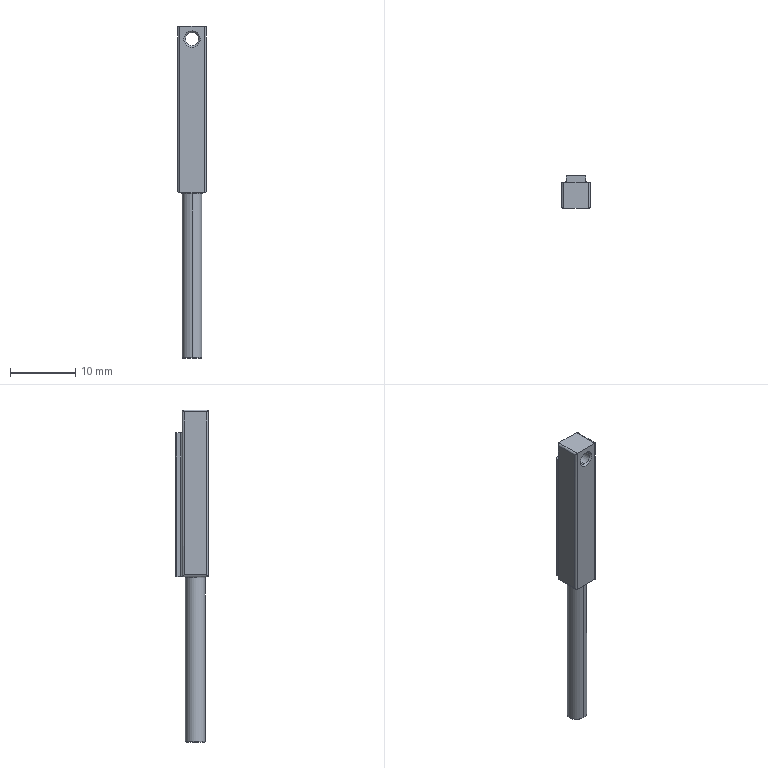Part | STEP file | Proximity switch AirTAC DS1-G-020-1 | 1 solid | 44 faces | box 4.4 x 5 x 50.8 mm | volume 677.466 mm3 | cylinder 21 | plane 15 | torus 4 | cone 4 | commonest cylinder face diameters 0.4 x8 0.6 x8 2.013 x2 3 x2 4.306 x1
STEP:
#1=CARTESIAN_POINT('',(0.,1.7,0.));
#2=VERTEX_POINT('',#1);
#3=CARTESIAN_POINT('',(0.,-1.7,0.));
#4=VERTEX_POINT('',#3);
#5=CARTESIAN_POINT('',(0.,0.,0.));
#6=DIRECTION('',(0.,0.,1.));
#7=DIRECTION('',(0.,-1.,0.));
#8=AXIS2_PLACEMENT_3D('',#5,#6,#7);
#9=CIRCLE('',#8,1.7);
#10=EDGE_CURVE('',#2,#4,#9,.T.);
#11=ORIENTED_EDGE('',*,*,#10,.F.);
#12=CARTESIAN_POINT('',(0.,1.5,-0.2));
#13=VERTEX_POINT('',#12);
#14=CARTESIAN_POINT('',(0.,1.7,-0.2));
#15=DIRECTION('',(1.,0.,0.));
#16=DIRECTION('',(0.,1.,0.));
#17=AXIS2_PLACEMENT_3D('',#14,#15,#16);
#18=CIRCLE('',#17,0.2);
#19=EDGE_CURVE('',#2,#13,#18,.T.);
#20=ORIENTED_EDGE('',*,*,#19,.T.);
#21=CARTESIAN_POINT('',(0.,-1.5,-0.2));
#22=VERTEX_POINT('',#21);
#23=CARTESIAN_POINT('',(0.,0.,-0.2));
#24=DIRECTION('',(0.,0.,1.));
#25=DIRECTION('',(0.,-1.,0.));
#26=AXIS2_PLACEMENT_3D('',#23,#24,#25);
#27=CIRCLE('',#26,1.5);
#28=EDGE_CURVE('',#13,#22,#27,.T.);
#29=ORIENTED_EDGE('',*,*,#28,.T.);
#30=CARTESIAN_POINT('',(0.,-1.7,-0.2));
#31=DIRECTION('',(-1.,0.,0.));
#32=DIRECTION('',(0.,0.,1.));
#33=AXIS2_PLACEMENT_3D('',#30,#31,#32);
#34=CIRCLE('',#33,0.2);
#35=EDGE_CURVE('',#4,#22,#34,.T.);
#36=ORIENTED_EDGE('',*,*,#35,.F.);
#37=EDGE_LOOP('',(#11,#20,#29,#36));
#38=FACE_OUTER_BOUND('',#37,.T.);
#39=CARTESIAN_POINT('',(0.,0.,-0.2));
#40=DIRECTION('',(0.,0.,1.));
#41=DIRECTION('',(0.,-1.,0.));
#42=AXIS2_PLACEMENT_3D('',#39,#40,#41);
#43=TOROIDAL_SURFACE('',#42,1.7,0.2);
#44=ADVANCED_FACE('',(#38),#43,.F.);
#45=CARTESIAN_POINT('',(0.,-1.5,-25.2));
#46=VERTEX_POINT('',#45);
#47=CARTESIAN_POINT('',(0.,1.5,-25.2));
#48=VERTEX_POINT('',#47);
#49=CARTESIAN_POINT('',(0.,0.,-25.2));
#50=DIRECTION('',(0.,0.,1.));
#51=DIRECTION('',(0.,-1.,0.));
#52=AXIS2_PLACEMENT_3D('',#49,#50,#51);
#53=CIRCLE('',#52,1.5);
#54=EDGE_CURVE('',#46,#48,#53,.T.);
#55=ORIENTED_EDGE('',*,*,#54,.T.);
#56=CARTESIAN_POINT('',(0.,1.5,-25.3));
#57=DIRECTION('',(0.,0.,1.));
#58=VECTOR('',#57,1000.);
#59=LINE('',#56,#58);
#60=EDGE_CURVE('',#48,#13,#59,.T.);
#61=ORIENTED_EDGE('',*,*,#60,.T.);
#62=CARTESIAN_POINT('',(0.,0.,-0.2));
#63=DIRECTION('',(0.,0.,1.));
#64=DIRECTION('',(0.,-1.,0.));
#65=AXIS2_PLACEMENT_3D('',#62,#63,#64);
#66=CIRCLE('',#65,1.5);
#67=EDGE_CURVE('',#22,#13,#66,.T.);
#68=ORIENTED_EDGE('',*,*,#67,.F.);
#69=CARTESIAN_POINT('',(0.,-1.5,-25.3));
#70=DIRECTION('',(0.,0.,1.));
#71=VECTOR('',#70,1000.);
#72=LINE('',#69,#71);
#73=EDGE_CURVE('',#46,#22,#72,.T.);
#74=ORIENTED_EDGE('',*,*,#73,.F.);
#75=EDGE_LOOP('',(#55,#61,#68,#74));
#76=FACE_OUTER_BOUND('',#75,.T.);
#77=CARTESIAN_POINT('',(0.,0.,-25.3));
#78=DIRECTION('',(0.,0.,1.));
#79=DIRECTION('',(0.,-1.,0.));
#80=AXIS2_PLACEMENT_3D('',#77,#78,#79);
#81=CYLINDRICAL_SURFACE('',#80,1.5);
#82=ADVANCED_FACE('',(#76),#81,.T.);
#83=CARTESIAN_POINT('',(0.,-1.4,-25.3));
#84=VERTEX_POINT('',#83);
#85=CARTESIAN_POINT('',(0.,1.4,-25.3));
#86=VERTEX_POINT('',#85);
#87=CARTESIAN_POINT('',(0.,0.,-25.3));
#88=DIRECTION('',(0.,0.,1.));
#89=DIRECTION('',(0.,-1.,0.));
#90=AXIS2_PLACEMENT_3D('',#87,#88,#89);
#91=CIRCLE('',#90,1.4);
#92=EDGE_CURVE('',#84,#86,#91,.T.);
#93=ORIENTED_EDGE('',*,*,#92,.T.);
#94=CARTESIAN_POINT('',(0.,1.4,-25.2));
#95=DIRECTION('',(1.,0.,0.));
#96=DIRECTION('',(0.,1.,0.));
#97=AXIS2_PLACEMENT_3D('',#94,#95,#96);
#98=CIRCLE('',#97,0.1);
#99=EDGE_CURVE('',#86,#48,#98,.T.);
#100=ORIENTED_EDGE('',*,*,#99,.T.);
#101=ORIENTED_EDGE('',*,*,#54,.F.);
#102=CARTESIAN_POINT('',(0.,-1.4,-25.2));
#103=DIRECTION('',(-1.,0.,0.));
#104=DIRECTION('',(0.,0.,1.));
#105=AXIS2_PLACEMENT_3D('',#102,#103,#104);
#106=CIRCLE('',#105,0.1);
#107=EDGE_CURVE('',#84,#46,#106,.T.);
#108=ORIENTED_EDGE('',*,*,#107,.F.);
#109=EDGE_LOOP('',(#93,#100,#101,#108));
#110=FACE_OUTER_BOUND('',#109,.T.);
#111=CARTESIAN_POINT('',(0.,0.,-25.2));
#112=DIRECTION('',(0.,0.,1.));
#113=DIRECTION('',(0.,-1.,0.));
#114=AXIS2_PLACEMENT_3D('',#111,#112,#113);
#115=TOROIDAL_SURFACE('',#114,1.4,0.1);
#116=ADVANCED_FACE('',(#110),#115,.T.);
#117=CARTESIAN_POINT('',(0.,1.756,24.506));
#118=VERTEX_POINT('',#117);
#119=CARTESIAN_POINT('',(0.,1.756,22.494));
#120=VERTEX_POINT('',#119);
#121=CARTESIAN_POINT('',(0.,1.756,23.5));
#122=DIRECTION('',(0.,-1.,0.));
#123=DIRECTION('',(0.,0.,-1.));
#124=AXIS2_PLACEMENT_3D('',#121,#122,#123);
#125=CIRCLE('',#124,1.007);
#126=EDGE_CURVE('',#118,#120,#125,.T.);
#127=ORIENTED_EDGE('',*,*,#126,.T.);
#128=CARTESIAN_POINT('',(0.,2.,22.25));
#129=VERTEX_POINT('',#128);
#130=CARTESIAN_POINT('',(0.,2.,22.25));
#131=DIRECTION('',(0.,0.7071,-0.7071));
#132=VECTOR('',#131,1000.);
#133=LINE('',#130,#132);
#134=EDGE_CURVE('',#120,#129,#133,.T.);
#135=ORIENTED_EDGE('',*,*,#134,.T.);
#136=CARTESIAN_POINT('',(0.,2.,24.75));
#137=VERTEX_POINT('',#136);
#138=CARTESIAN_POINT('',(0.,2.,23.5));
#139=DIRECTION('',(0.,-1.,0.));
#140=DIRECTION('',(0.,0.,-1.));
#141=AXIS2_PLACEMENT_3D('',#138,#139,#140);
#142=CIRCLE('',#141,1.25);
#143=EDGE_CURVE('',#137,#129,#142,.T.);
#144=ORIENTED_EDGE('',*,*,#143,.F.);
#145=CARTESIAN_POINT('',(0.,2.,24.75));
#146=DIRECTION('',(0.,0.7071,0.7071));
#147=VECTOR('',#146,1000.);
#148=LINE('',#145,#147);
#149=EDGE_CURVE('',#118,#137,#148,.T.);
#150=ORIENTED_EDGE('',*,*,#149,.F.);
#151=EDGE_LOOP('',(#127,#135,#144,#150));
#152=FACE_OUTER_BOUND('',#151,.T.);
#153=CARTESIAN_POINT('',(0.,2.,23.5));
#154=DIRECTION('',(0.,1.,0.));
#155=DIRECTION('',(0.,0.,1.));
#156=AXIS2_PLACEMENT_3D('',#153,#154,#155);
#157=CONICAL_SURFACE('',#156,1.25,0.7854);
#158=ADVANCED_FACE('',(#152),#157,.F.);
#159=ORIENTED_EDGE('',*,*,#126,.F.);
#160=CARTESIAN_POINT('',(0.,-1.756,24.506));
#161=VERTEX_POINT('',#160);
#162=CARTESIAN_POINT('',(0.,2.,24.506));
#163=DIRECTION('',(0.,-1.,0.));
#164=VECTOR('',#163,1000.);
#165=LINE('',#162,#164);
#166=EDGE_CURVE('',#118,#161,#165,.T.);
#167=ORIENTED_EDGE('',*,*,#166,.T.);
#168=CARTESIAN_POINT('',(0.,-1.756,22.494));
#169=VERTEX_POINT('',#168);
#170=CARTESIAN_POINT('',(0.,-1.756,23.5));
#171=DIRECTION('',(0.,-1.,0.));
#172=DIRECTION('',(0.,0.,-1.));
#173=AXIS2_PLACEMENT_3D('',#170,#171,#172);
#174=CIRCLE('',#173,1.007);
#175=EDGE_CURVE('',#161,#169,#174,.T.);
#176=ORIENTED_EDGE('',*,*,#175,.T.);
#177=CARTESIAN_POINT('',(0.,2.,22.494));
#178=DIRECTION('',(0.,-1.,0.));
#179=VECTOR('',#178,1000.);
#180=LINE('',#177,#179);
#181=EDGE_CURVE('',#120,#169,#180,.T.);
#182=ORIENTED_EDGE('',*,*,#181,.F.);
#183=EDGE_LOOP('',(#159,#167,#176,#182));
#184=FACE_OUTER_BOUND('',#183,.T.);
#185=CARTESIAN_POINT('',(0.,2.,23.5));
#186=DIRECTION('',(0.,-1.,0.));
#187=DIRECTION('',(0.,0.,-1.));
#188=AXIS2_PLACEMENT_3D('',#185,#186,#187);
#189=CYLINDRICAL_SURFACE('',#188,1.007);
#190=ADVANCED_FACE('',(#184),#189,.F.);
#191=ORIENTED_EDGE('',*,*,#175,.F.);
#192=CARTESIAN_POINT('',(0.,-2.,24.75));
#193=VERTEX_POINT('',#192);
#194=CARTESIAN_POINT('',(0.,-1.756,24.506));
#195=DIRECTION('',(0.,-0.7071,0.7071));
#196=VECTOR('',#195,1000.);
#197=LINE('',#194,#196);
#198=EDGE_CURVE('',#161,#193,#197,.T.);
#199=ORIENTED_EDGE('',*,*,#198,.T.);
#200=CARTESIAN_POINT('',(0.,-2.,22.25));
#201=VERTEX_POINT('',#200);
#202=CARTESIAN_POINT('',(0.,-2.,23.5));
#203=DIRECTION('',(0.,-1.,0.));
#204=DIRECTION('',(0.,0.,-1.));
#205=AXIS2_PLACEMENT_3D('',#202,#203,#204);
#206=CIRCLE('',#205,1.25);
#207=EDGE_CURVE('',#193,#201,#206,.T.);
#208=ORIENTED_EDGE('',*,*,#207,.T.);
#209=CARTESIAN_POINT('',(0.,-1.756,22.494));
#210=DIRECTION('',(0.,-0.7071,-0.7071));
#211=VECTOR('',#210,1000.);
#212=LINE('',#209,#211);
#213=EDGE_CURVE('',#169,#201,#212,.T.);
#214=ORIENTED_EDGE('',*,*,#213,.F.);
#215=EDGE_LOOP('',(#191,#199,#208,#214));
#216=FACE_OUTER_BOUND('',#215,.T.);
#217=CARTESIAN_POINT('',(0.,-1.756,23.5));
#218=DIRECTION('',(0.,-1.,0.));
#219=DIRECTION('',(0.,0.,-1.));
#220=AXIS2_PLACEMENT_3D('',#217,#218,#219);
#221=CONICAL_SURFACE('',#220,1.007,0.7854);
#222=ADVANCED_FACE('',(#216),#221,.F.);
#223=CARTESIAN_POINT('',(-1.9,-2.,0.));
#224=VERTEX_POINT('',#223);
#225=CARTESIAN_POINT('',(1.9,-2.,0.));
#226=VERTEX_POINT('',#225);
#227=CARTESIAN_POINT('',(-1.9,-2.,0.));
#228=DIRECTION('',(1.,0.,0.));
#229=VECTOR('',#228,1000.);
#230=LINE('',#227,#229);
#231=EDGE_CURVE('',#224,#226,#230,.T.);
#232=ORIENTED_EDGE('',*,*,#231,.T.);
#233=CARTESIAN_POINT('',(1.9,-2.,25.5));
#234=VERTEX_POINT('',#233);
#235=CARTESIAN_POINT('',(1.9,-2.,25.5));
#236=DIRECTION('',(0.,0.,-1.));
#237=VECTOR('',#236,1000.);
#238=LINE('',#235,#237);
#239=EDGE_CURVE('',#234,#226,#238,.T.);
#240=ORIENTED_EDGE('',*,*,#239,.F.);
#241=CARTESIAN_POINT('',(-1.9,-2.,25.5));
#242=VERTEX_POINT('',#241);
#243=CARTESIAN_POINT('',(-1.9,-2.,25.5));
#244=DIRECTION('',(1.,0.,0.));
#245=VECTOR('',#244,1000.);
#246=LINE('',#243,#245);
#247=EDGE_CURVE('',#242,#234,#246,.T.);
#248=ORIENTED_EDGE('',*,*,#247,.F.);
#249=CARTESIAN_POINT('',(-1.9,-2.,25.5));
#250=DIRECTION('',(0.,0.,-1.));
#251=VECTOR('',#250,1000.);
#252=LINE('',#249,#251);
#253=EDGE_CURVE('',#242,#224,#252,.T.);
#254=ORIENTED_EDGE('',*,*,#253,.T.);
#255=EDGE_LOOP('',(#232,#240,#248,#254));
#256=FACE_OUTER_BOUND('',#255,.T.);
#257=CARTESIAN_POINT('',(0.,-2.,23.5));
#258=DIRECTION('',(0.,-1.,0.));
#259=DIRECTION('',(0.,0.,-1.));
#260=AXIS2_PLACEMENT_3D('',#257,#258,#259);
#261=CIRCLE('',#260,1.25);
#262=EDGE_CURVE('',#201,#193,#261,.T.);
#263=ORIENTED_EDGE('',*,*,#262,.F.);
#264=ORIENTED_EDGE('',*,*,#207,.F.);
#265=EDGE_LOOP('',(#263,#264));
#266=FACE_BOUND('',#265,.T.);
#267=CARTESIAN_POINT('',(-1.9,-2.,25.5));
#268=DIRECTION('',(0.,1.,0.));
#269=DIRECTION('',(0.,0.,1.));
#270=AXIS2_PLACEMENT_3D('',#267,#268,#269);
#271=PLANE('',#270);
#272=ADVANCED_FACE('',(#256,#266),#271,.F.);
#273=CARTESIAN_POINT('',(-1.7,2.,0.));
#274=VERTEX_POINT('',#273);
#275=CARTESIAN_POINT('',(-1.9,2.,0.));
#276=VERTEX_POINT('',#275);
#277=CARTESIAN_POINT('',(-1.7,2.,0.));
#278=DIRECTION('',(-1.,0.,0.));
#279=VECTOR('',#278,1000.);
#280=LINE('',#277,#279);
#281=EDGE_CURVE('',#274,#276,#280,.T.);
#282=ORIENTED_EDGE('',*,*,#281,.T.);
#283=CARTESIAN_POINT('',(-1.9,2.,25.5));
#284=VERTEX_POINT('',#283);
#285=CARTESIAN_POINT('',(-1.9,2.,25.5));
#286=DIRECTION('',(0.,0.,-1.));
#287=VECTOR('',#286,1000.);
#288=LINE('',#285,#287);
#289=EDGE_CURVE('',#284,#276,#288,.T.);
#290=ORIENTED_EDGE('',*,*,#289,.F.);
#291=CARTESIAN_POINT('',(1.9,2.,25.5));
#292=VERTEX_POINT('',#291);
#293=CARTESIAN_POINT('',(1.9,2.,25.5));
#294=DIRECTION('',(-1.,0.,0.));
#295=VECTOR('',#294,1000.);
#296=LINE('',#293,#295);
#297=EDGE_CURVE('',#292,#284,#296,.T.);
#298=ORIENTED_EDGE('',*,*,#297,.F.);
#299=CARTESIAN_POINT('',(1.9,2.,0.));
#300=VERTEX_POINT('',#299);
#301=CARTESIAN_POINT('',(1.9,2.,25.5));
#302=DIRECTION('',(0.,0.,-1.));
#303=VECTOR('',#302,1000.);
#304=LINE('',#301,#303);
#305=EDGE_CURVE('',#292,#300,#304,.T.);
#306=ORIENTED_EDGE('',*,*,#305,.T.);
#307=CARTESIAN_POINT('',(1.7,2.,0.));
#308=VERTEX_POINT('',#307);
#309=CARTESIAN_POINT('',(1.9,2.,0.));
#310=DIRECTION('',(-1.,0.,0.));
#311=VECTOR('',#310,1000.);
#312=LINE('',#309,#311);
#313=EDGE_CURVE('',#300,#308,#312,.T.);
#314=ORIENTED_EDGE('',*,*,#313,.T.);
#315=CARTESIAN_POINT('',(1.7,2.,22.));
#316=VERTEX_POINT('',#315);
#317=CARTESIAN_POINT('',(1.7,2.,25.5));
#318=DIRECTION('',(0.,0.,-1.));
#319=VECTOR('',#318,1000.);
#320=LINE('',#317,#319);
#321=EDGE_CURVE('',#316,#308,#320,.T.);
#322=ORIENTED_EDGE('',*,*,#321,.F.);
#323=CARTESIAN_POINT('',(-1.7,2.,22.));
#324=VERTEX_POINT('',#323);
#325=CARTESIAN_POINT('',(-2.2,2.,22.));
#326=DIRECTION('',(1.,0.,0.));
#327=VECTOR('',#326,1000.);
#328=LINE('',#325,#327);
#329=EDGE_CURVE('',#324,#316,#328,.T.);
#330=ORIENTED_EDGE('',*,*,#329,.F.);
#331=CARTESIAN_POINT('',(-1.7,2.,25.5));
#332=DIRECTION('',(0.,0.,-1.));
#333=VECTOR('',#332,1000.);
#334=LINE('',#331,#333);
#335=EDGE_CURVE('',#324,#274,#334,.T.);
#336=ORIENTED_EDGE('',*,*,#335,.T.);
#337=EDGE_LOOP('',(#282,#290,#298,#306,#314,#322,#330,#336));
#338=FACE_OUTER_BOUND('',#337,.T.);
#339=ORIENTED_EDGE('',*,*,#143,.T.);
#340=CARTESIAN_POINT('',(0.,2.,23.5));
#341=DIRECTION('',(0.,-1.,0.));
#342=DIRECTION('',(0.,0.,-1.));
#343=AXIS2_PLACEMENT_3D('',#340,#341,#342);
#344=CIRCLE('',#343,1.25);
#345=EDGE_CURVE('',#129,#137,#344,.T.);
#346=ORIENTED_EDGE('',*,*,#345,.T.);
#347=EDGE_LOOP('',(#339,#346));
#348=FACE_BOUND('',#347,.T.);
#349=CARTESIAN_POINT('',(-1.7,2.,25.5));
#350=DIRECTION('',(0.,-1.,0.));
#351=DIRECTION('',(0.,0.,-1.));
#352=AXIS2_PLACEMENT_3D('',#349,#350,#351);
#353=PLANE('',#352);
#354=ADVANCED_FACE('',(#338,#348),#353,.F.);
#355=CARTESIAN_POINT('',(-2.2,-1.7,25.2));
#356=VERTEX_POINT('',#355);
#357=CARTESIAN_POINT('',(-2.2,-1.7,25.2));
#358=CARTESIAN_POINT('',(-2.2,-1.876,25.376));
#359=CARTESIAN_POINT('',(-2.076,-2.,25.5));
#360=CARTESIAN_POINT('',(-1.9,-2.,25.5));
#361=(BOUNDED_CURVE()B_SPLINE_CURVE(3,(#357,#358,#359,#360),.UNSPECIFIED.,.F.,.F.)B_SPLINE_CURVE_WITH_KNOTS((4,4),(1.571,3.142),.UNSPECIFIED.)CURVE()GEOMETRIC_REPRESENTATION_ITEM()RATIONAL_B_SPLINE_CURVE((1.,0.8047,0.8047,1.))REPRESENTATION_ITEM(''));
#362=EDGE_CURVE('',#356,#242,#361,.T.);
#363=ORIENTED_EDGE('',*,*,#362,.F.);
#364=CARTESIAN_POINT('',(-2.2,-1.7,0.3));
#365=VERTEX_POINT('',#364);
#366=CARTESIAN_POINT('',(-2.2,-1.7,25.5));
#367=DIRECTION('',(0.,0.,-1.));
#368=VECTOR('',#367,1000.);
#369=LINE('',#366,#368);
#370=EDGE_CURVE('',#356,#365,#369,.T.);
#371=ORIENTED_EDGE('',*,*,#370,.T.);
#372=CARTESIAN_POINT('',(-1.9,-2.,0.));
#373=CARTESIAN_POINT('',(-2.076,-2.,0.));
#374=CARTESIAN_POINT('',(-2.2,-1.876,0.1243));
#375=CARTESIAN_POINT('',(-2.2,-1.7,0.3));
#376=(BOUNDED_CURVE()B_SPLINE_CURVE(3,(#372,#373,#374,#375),.UNSPECIFIED.,.F.,.T.)B_SPLINE_CURVE_WITH_KNOTS((4,4),(0.,1.571),.UNSPECIFIED.)CURVE()GEOMETRIC_REPRESENTATION_ITEM()RATIONAL_B_SPLINE_CURVE((1.,0.8047,0.8047,1.))REPRESENTATION_ITEM(''));
#377=EDGE_CURVE('',#224,#365,#376,.T.);
#378=ORIENTED_EDGE('',*,*,#377,.F.);
#379=ORIENTED_EDGE('',*,*,#253,.F.);
#380=EDGE_LOOP('',(#363,#371,#378,#379));
#381=FACE_OUTER_BOUND('',#380,.T.);
#382=CARTESIAN_POINT('',(-1.9,-1.7,25.5));
#383=DIRECTION('',(0.,0.,-1.));
#384=DIRECTION('',(-1.,0.,0.));
#385=AXIS2_PLACEMENT_3D('',#382,#383,#384);
#386=CYLINDRICAL_SURFACE('',#385,0.3);
#387=ADVANCED_FACE('',(#381),#386,.T.);
#388=CARTESIAN_POINT('',(2.2,-1.7,0.3));
#389=VERTEX_POINT('',#388);
#390=CARTESIAN_POINT('',(2.2,-1.7,0.3));
#391=CARTESIAN_POINT('',(2.2,-1.876,0.1243));
#392=CARTESIAN_POINT('',(2.076,-2.,0.));
#393=CARTESIAN_POINT('',(1.9,-2.,0.));
#394=(BOUNDED_CURVE()B_SPLINE_CURVE(3,(#390,#391,#392,#393),.UNSPECIFIED.,.F.,.F.)B_SPLINE_CURVE_WITH_KNOTS((4,4),(4.712,6.283),.UNSPECIFIED.)CURVE()GEOMETRIC_REPRESENTATION_ITEM()RATIONAL_B_SPLINE_CURVE((1.,0.8047,0.8047,1.))REPRESENTATION_ITEM(''));
#395=EDGE_CURVE('',#389,#226,#394,.T.);
#396=ORIENTED_EDGE('',*,*,#395,.F.);
#397=CARTESIAN_POINT('',(2.2,-1.7,25.2));
#398=VERTEX_POINT('',#397);
#399=CARTESIAN_POINT('',(2.2,-1.7,25.5));
#400=DIRECTION('',(0.,0.,-1.));
#401=VECTOR('',#400,1000.);
#402=LINE('',#399,#401);
#403=EDGE_CURVE('',#398,#389,#402,.T.);
#404=ORIENTED_EDGE('',*,*,#403,.F.);
#405=CARTESIAN_POINT('',(1.9,-2.,25.5));
#406=CARTESIAN_POINT('',(2.076,-2.,25.5));
#407=CARTESIAN_POINT('',(2.2,-1.876,25.376));
#408=CARTESIAN_POINT('',(2.2,-1.7,25.2));
#409=(BOUNDED_CURVE()B_SPLINE_CURVE(3,(#405,#406,#407,#408),.UNSPECIFIED.,.F.,.F.)B_SPLINE_CURVE_WITH_KNOTS((4,4),(3.142,4.712),.UNSPECIFIED.)CURVE()GEOMETRIC_REPRESENTATION_ITEM()RATIONAL_B_SPLINE_CURVE((1.,0.8047,0.8047,1.))REPRESENTATION_ITEM(''));
#410=EDGE_CURVE('',#234,#398,#409,.T.);
#411=ORIENTED_EDGE('',*,*,#410,.F.);
#412=ORIENTED_EDGE('',*,*,#239,.T.);
#413=EDGE_LOOP('',(#396,#404,#411,#412));
#414=FACE_OUTER_BOUND('',#413,.T.);
#415=CARTESIAN_POINT('',(1.9,-1.7,25.5));
#416=DIRECTION('',(0.,0.,-1.));
#417=DIRECTION('',(-1.,0.,0.));
#418=AXIS2_PLACEMENT_3D('',#415,#416,#417);
#419=CYLINDRICAL_SURFACE('',#418,0.3);
#420=ADVANCED_FACE('',(#414),#419,.T.);
#421=ORIENTED_EDGE('',*,*,#403,.T.);
#422=CARTESIAN_POINT('',(2.2,1.7,0.3));
#423=VERTEX_POINT('',#422);
#424=CARTESIAN_POINT('',(2.2,-5.,0.3));
#425=DIRECTION('',(0.,1.,0.));
#426=VECTOR('',#425,1000.);
#427=LINE('',#424,#426);
#428=EDGE_CURVE('',#389,#423,#427,.T.);
#429=ORIENTED_EDGE('',*,*,#428,.T.);
#430=CARTESIAN_POINT('',(2.2,1.7,25.2));
#431=VERTEX_POINT('',#430);
#432=CARTESIAN_POINT('',(2.2,1.7,25.5));
#433=DIRECTION('',(0.,0.,-1.));
#434=VECTOR('',#433,1000.);
#435=LINE('',#432,#434);
#436=EDGE_CURVE('',#431,#423,#435,.T.);
#437=ORIENTED_EDGE('',*,*,#436,.F.);
#438=CARTESIAN_POINT('',(2.2,-5.,25.2));
#439=DIRECTION('',(0.,1.,0.));
#440=VECTOR('',#439,1000.);
#441=LINE('',#438,#440);
#442=EDGE_CURVE('',#398,#431,#441,.T.);
#443=ORIENTED_EDGE('',*,*,#442,.F.);
#444=EDGE_LOOP('',(#421,#429,#437,#443));
#445=FACE_OUTER_BOUND('',#444,.T.);
#446=CARTESIAN_POINT('',(2.2,-1.7,25.5));
#447=DIRECTION('',(-1.,0.,0.));
#448=DIRECTION('',(0.,0.,1.));
#449=AXIS2_PLACEMENT_3D('',#446,#447,#448);
#450=PLANE('',#449);
#451=ADVANCED_FACE('',(#445),#450,.F.);
#452=CARTESIAN_POINT('',(1.9,2.,0.));
#453=CARTESIAN_POINT('',(2.076,2.,0.));
#454=CARTESIAN_POINT('',(2.2,1.876,0.1243));
#455=CARTESIAN_POINT('',(2.2,1.7,0.3));
#456=(BOUNDED_CURVE()B_SPLINE_CURVE(3,(#452,#453,#454,#455),.UNSPECIFIED.,.F.,.F.)B_SPLINE_CURVE_WITH_KNOTS((4,4),(0.,1.571),.UNSPECIFIED.)CURVE()GEOMETRIC_REPRESENTATION_ITEM()RATIONAL_B_SPLINE_CURVE((1.,0.8047,0.8047,1.))REPRESENTATION_ITEM(''));
#457=EDGE_CURVE('',#300,#423,#456,.T.);
#458=ORIENTED_EDGE('',*,*,#457,.F.);
#459=ORIENTED_EDGE('',*,*,#305,.F.);
#460=CARTESIAN_POINT('',(2.2,1.7,25.2));
#461=CARTESIAN_POINT('',(2.2,1.876,25.376));
#462=CARTESIAN_POINT('',(2.076,2.,25.5));
#463=CARTESIAN_POINT('',(1.9,2.,25.5));
#464=(BOUNDED_CURVE()B_SPLINE_CURVE(3,(#460,#461,#462,#463),.UNSPECIFIED.,.F.,.F.)B_SPLINE_CURVE_WITH_KNOTS((4,4),(1.571,3.142),.UNSPECIFIED.)CURVE()GEOMETRIC_REPRESENTATION_ITEM()RATIONAL_B_SPLINE_CURVE((1.,0.8047,0.8047,1.))REPRESENTATION_ITEM(''));
#465=EDGE_CURVE('',#431,#292,#464,.T.);
#466=ORIENTED_EDGE('',*,*,#465,.F.);
#467=ORIENTED_EDGE('',*,*,#436,.T.);
#468=EDGE_LOOP('',(#458,#459,#466,#467));
#469=FACE_OUTER_BOUND('',#468,.T.);
#470=CARTESIAN_POINT('',(1.9,1.7,25.5));
#471=DIRECTION('',(0.,0.,-1.));
#472=DIRECTION('',(-1.,0.,0.));
#473=AXIS2_PLACEMENT_3D('',#470,#471,#472);
#474=CYLINDRICAL_SURFACE('',#473,0.3);
#475=ADVANCED_FACE('',(#469),#474,.T.);
#476=CARTESIAN_POINT('',(-2.2,1.7,25.2));
#477=VERTEX_POINT('',#476);
#478=CARTESIAN_POINT('',(-1.9,2.,25.5));
#479=CARTESIAN_POINT('',(-2.076,2.,25.5));
#480=CARTESIAN_POINT('',(-2.2,1.876,25.376));
#481=CARTESIAN_POINT('',(-2.2,1.7,25.2));
#482=(BOUNDED_CURVE()B_SPLINE_CURVE(3,(#478,#479,#480,#481),.UNSPECIFIED.,.F.,.F.)B_SPLINE_CURVE_WITH_KNOTS((4,4),(3.142,4.712),.UNSPECIFIED.)CURVE()GEOMETRIC_REPRESENTATION_ITEM()RATIONAL_B_SPLINE_CURVE((1.,0.8047,0.8047,1.))REPRESENTATION_ITEM(''));
#483=EDGE_CURVE('',#284,#477,#482,.T.);
#484=ORIENTED_EDGE('',*,*,#483,.F.);
#485=ORIENTED_EDGE('',*,*,#289,.T.);
#486=CARTESIAN_POINT('',(-2.2,1.7,0.3));
#487=VERTEX_POINT('',#486);
#488=CARTESIAN_POINT('',(-2.2,1.7,0.3));
#489=CARTESIAN_POINT('',(-2.2,1.876,0.1243));
#490=CARTESIAN_POINT('',(-2.076,2.,0.));
#491=CARTESIAN_POINT('',(-1.9,2.,0.));
#492=(BOUNDED_CURVE()B_SPLINE_CURVE(3,(#488,#489,#490,#491),.UNSPECIFIED.,.F.,.F.)B_SPLINE_CURVE_WITH_KNOTS((4,4),(4.712,6.283),.UNSPECIFIED.)CURVE()GEOMETRIC_REPRESENTATION_ITEM()RATIONAL_B_SPLINE_CURVE((1.,0.8047,0.8047,1.))REPRESENTATION_ITEM(''));
#493=EDGE_CURVE('',#487,#276,#492,.T.);
#494=ORIENTED_EDGE('',*,*,#493,.F.);
#495=CARTESIAN_POINT('',(-2.2,1.7,25.5));
#496=DIRECTION('',(0.,0.,-1.));
#497=VECTOR('',#496,1000.);
#498=LINE('',#495,#497);
#499=EDGE_CURVE('',#477,#487,#498,.T.);
#500=ORIENTED_EDGE('',*,*,#499,.F.);
#501=EDGE_LOOP('',(#484,#485,#494,#500));
#502=FACE_OUTER_BOUND('',#501,.T.);
#503=CARTESIAN_POINT('',(-1.9,1.7,25.5));
#504=DIRECTION('',(0.,0.,-1.));
#505=DIRECTION('',(-1.,0.,0.));
#506=AXIS2_PLACEMENT_3D('',#503,#504,#505);
#507=CYLINDRICAL_SURFACE('',#506,0.3);
#508=ADVANCED_FACE('',(#502),#507,.T.);
#509=ORIENTED_EDGE('',*,*,#370,.F.);
#510=CARTESIAN_POINT('',(-2.2,-5.,25.2));
#511=DIRECTION('',(0.,1.,0.));
#512=VECTOR('',#511,1000.);
#513=LINE('',#510,#512);
#514=EDGE_CURVE('',#356,#477,#513,.T.);
#515=ORIENTED_EDGE('',*,*,#514,.T.);
#516=ORIENTED_EDGE('',*,*,#499,.T.);
#517=CARTESIAN_POINT('',(-2.2,-5.,0.3));
#518=DIRECTION('',(0.,1.,0.));
#519=VECTOR('',#518,1000.);
#520=LINE('',#517,#519);
#521=EDGE_CURVE('',#365,#487,#520,.T.);
#522=ORIENTED_EDGE('',*,*,#521,.F.);
#523=EDGE_LOOP('',(#509,#515,#516,#522));
#524=FACE_OUTER_BOUND('',#523,.T.);
#525=CARTESIAN_POINT('',(-2.2,1.7,25.5));
#526=DIRECTION('',(1.,0.,0.));
#527=DIRECTION('',(0.,0.,-1.));
#528=AXIS2_PLACEMENT_3D('',#525,#526,#527);
#529=PLANE('',#528);
#530=ADVANCED_FACE('',(#524),#529,.F.);
#531=CARTESIAN_POINT('',(-1.9,-5.,25.5));
#532=DIRECTION('',(0.,1.,0.));
#533=VECTOR('',#532,1000.);
#534=LINE('',#531,#533);
#535=EDGE_CURVE('',#242,#284,#534,.T.);
#536=ORIENTED_EDGE('',*,*,#535,.F.);
#537=ORIENTED_EDGE('',*,*,#247,.T.);
#538=CARTESIAN_POINT('',(1.9,-5.,25.5));
#539=DIRECTION('',(0.,1.,0.));
#540=VECTOR('',#539,1000.);
#541=LINE('',#538,#540);
#542=EDGE_CURVE('',#234,#292,#541,.T.);
#543=ORIENTED_EDGE('',*,*,#542,.T.);
#544=ORIENTED_EDGE('',*,*,#297,.T.);
#545=EDGE_LOOP('',(#536,#537,#543,#544));
#546=FACE_OUTER_BOUND('',#545,.T.);
#547=CARTESIAN_POINT('',(-1.9,-1.7,25.5));
#548=DIRECTION('',(0.,0.,1.));
#549=DIRECTION('',(1.,0.,0.));
#550=AXIS2_PLACEMENT_3D('',#547,#548,#549);
#551=PLANE('',#550);
#552=ADVANCED_FACE('',(#546),#551,.T.);
#553=CARTESIAN_POINT('',(0.,0.,0.));
#554=DIRECTION('',(0.,0.,1.));
#555=DIRECTION('',(0.,-1.,0.));
#556=AXIS2_PLACEMENT_3D('',#553,#554,#555);
#557=CIRCLE('',#556,1.7);
#558=EDGE_CURVE('',#4,#2,#557,.T.);
#559=ORIENTED_EDGE('',*,*,#558,.T.);
#560=ORIENTED_EDGE('',*,*,#10,.T.);
#561=EDGE_LOOP('',(#559,#560));
#562=FACE_BOUND('',#561,.T.);
#563=ORIENTED_EDGE('',*,*,#231,.F.);
#564=CARTESIAN_POINT('',(-1.9,-5.,0.));
#565=DIRECTION('',(0.,1.,0.));
#566=VECTOR('',#565,1000.);
#567=LINE('',#564,#566);
#568=EDGE_CURVE('',#224,#276,#567,.T.);
#569=ORIENTED_EDGE('',*,*,#568,.T.);
#570=ORIENTED_EDGE('',*,*,#281,.F.);
#571=CARTESIAN_POINT('',(-1.5,2.2,0.));
#572=VERTEX_POINT('',#571);
#573=CARTESIAN_POINT('',(-1.7,2.2,0.));
#574=DIRECTION('',(0.,0.,-1.));
#575=DIRECTION('',(-1.,0.,0.));
#576=AXIS2_PLACEMENT_3D('',#573,#574,#575);
#577=CIRCLE('',#576,0.2);
#578=EDGE_CURVE('',#572,#274,#577,.T.);
#579=ORIENTED_EDGE('',*,*,#578,.F.);
#580=CARTESIAN_POINT('',(-1.5,2.8,0.));
#581=VERTEX_POINT('',#580);
#582=CARTESIAN_POINT('',(-1.5,2.8,0.));
#583=DIRECTION('',(0.,-1.,0.));
#584=VECTOR('',#583,1000.);
#585=LINE('',#582,#584);
#586=EDGE_CURVE('',#581,#572,#585,.T.);
#587=ORIENTED_EDGE('',*,*,#586,.F.);
#588=CARTESIAN_POINT('',(-1.3,3.,0.));
#589=VERTEX_POINT('',#588);
#590=CARTESIAN_POINT('',(-1.3,2.8,0.));
#591=DIRECTION('',(0.,0.,1.));
#592=DIRECTION('',(1.,0.,0.));
#593=AXIS2_PLACEMENT_3D('',#590,#591,#592);
#594=CIRCLE('',#593,0.2);
#595=EDGE_CURVE('',#589,#581,#594,.T.);
#596=ORIENTED_EDGE('',*,*,#595,.F.);
#597=CARTESIAN_POINT('',(1.3,3.,0.));
#598=VERTEX_POINT('',#597);
#599=CARTESIAN_POINT('',(1.3,3.,0.));
#600=DIRECTION('',(-1.,0.,0.));
#601=VECTOR('',#600,1000.);
#602=LINE('',#599,#601);
#603=EDGE_CURVE('',#598,#589,#602,.T.);
#604=ORIENTED_EDGE('',*,*,#603,.F.);
#605=CARTESIAN_POINT('',(1.5,2.8,0.));
#606=VERTEX_POINT('',#605);
#607=CARTESIAN_POINT('',(1.3,2.8,0.));
#608=DIRECTION('',(0.,0.,1.));
#609=DIRECTION('',(1.,0.,0.));
#610=AXIS2_PLACEMENT_3D('',#607,#608,#609);
#611=CIRCLE('',#610,0.2);
#612=EDGE_CURVE('',#606,#598,#611,.T.);
#613=ORIENTED_EDGE('',*,*,#612,.F.);
#614=CARTESIAN_POINT('',(1.5,2.2,0.));
#615=VERTEX_POINT('',#614);
#616=CARTESIAN_POINT('',(1.5,2.2,0.));
#617=DIRECTION('',(0.,1.,0.));
#618=VECTOR('',#617,1000.);
#619=LINE('',#616,#618);
#620=EDGE_CURVE('',#615,#606,#619,.T.);
#621=ORIENTED_EDGE('',*,*,#620,.F.);
#622=CARTESIAN_POINT('',(1.7,2.2,0.));
#623=DIRECTION('',(0.,0.,-1.));
#624=DIRECTION('',(-1.,0.,0.));
#625=AXIS2_PLACEMENT_3D('',#622,#623,#624);
#626=CIRCLE('',#625,0.2);
#627=EDGE_CURVE('',#308,#615,#626,.T.);
#628=ORIENTED_EDGE('',*,*,#627,.F.);
#629=ORIENTED_EDGE('',*,*,#313,.F.);
#630=CARTESIAN_POINT('',(1.9,-5.,0.));
#631=DIRECTION('',(0.,1.,0.));
#632=VECTOR('',#631,1000.);
#633=LINE('',#630,#632);
#634=EDGE_CURVE('',#226,#300,#633,.T.);
#635=ORIENTED_EDGE('',*,*,#634,.F.);
#636=EDGE_LOOP('',(#563,#569,#570,#579,#587,#596,#604,#613,#621,#628,#629,#635));
#637=FACE_OUTER_BOUND('',#636,.T.);
#638=CARTESIAN_POINT('',(-1.9,-1.7,0.));
#639=DIRECTION('',(0.,0.,1.));
#640=DIRECTION('',(1.,0.,0.));
#641=AXIS2_PLACEMENT_3D('',#638,#639,#640);
#642=PLANE('',#641);
#643=ADVANCED_FACE('',(#562,#637),#642,.F.);
#644=CARTESIAN_POINT('',(-0.75,2.627,18.3));
#645=VERTEX_POINT('',#644);
#646=CARTESIAN_POINT('',(-0.55,2.5,18.5));
#647=VERTEX_POINT('',#646);
#648=CARTESIAN_POINT('',(-0.75,2.627,18.3));
#649=CARTESIAN_POINT('',(-0.75,2.598,18.35));
#650=CARTESIAN_POINT('',(-0.7316,2.569,18.398));
#651=CARTESIAN_POINT('',(-0.6618,2.519,18.474));
#652=CARTESIAN_POINT('',(-0.608,2.5,18.5));
#653=CARTESIAN_POINT('',(-0.55,2.5,18.5));
#654=B_SPLINE_CURVE_WITH_KNOTS('',3,(#648,#649,#650,#651,#652,#653),.UNSPECIFIED.,.F.,.F.,(4,2,4),(0.,0.0001698,0.0003395),.UNSPECIFIED.);
#655=EDGE_CURVE('',#645,#647,#654,.T.);
#656=ORIENTED_EDGE('',*,*,#655,.F.);
#657=CARTESIAN_POINT('',(-0.75,3.,18.3));
#658=VERTEX_POINT('',#657);
#659=CARTESIAN_POINT('',(-0.75,1.,18.3));
#660=DIRECTION('',(0.,1.,0.));
#661=VECTOR('',#660,1000.);
#662=LINE('',#659,#661);
#663=EDGE_CURVE('',#645,#658,#662,.T.);
#664=ORIENTED_EDGE('',*,*,#663,.T.);
#665=CARTESIAN_POINT('',(-0.55,3.,18.5));
#666=VERTEX_POINT('',#665);
#667=CARTESIAN_POINT('',(-0.55,3.,18.3));
#668=DIRECTION('',(0.,1.,0.));
#669=DIRECTION('',(0.,0.,1.));
#670=AXIS2_PLACEMENT_3D('',#667,#668,#669);
#671=CIRCLE('',#670,0.2);
#672=EDGE_CURVE('',#658,#666,#671,.T.);
#673=ORIENTED_EDGE('',*,*,#672,.T.);
#674=CARTESIAN_POINT('',(-0.55,1.,18.5));
#675=DIRECTION('',(0.,1.,0.));
#676=VECTOR('',#675,1000.);
#677=LINE('',#674,#676);
#678=EDGE_CURVE('',#647,#666,#677,.T.);
#679=ORIENTED_EDGE('',*,*,#678,.F.);
#680=EDGE_LOOP('',(#656,#664,#673,#679));
#681=FACE_OUTER_BOUND('',#680,.T.);
#682=CARTESIAN_POINT('',(-0.55,1.,18.3));
#683=DIRECTION('',(0.,1.,0.));
#684=DIRECTION('',(0.,0.,1.));
#685=AXIS2_PLACEMENT_3D('',#682,#683,#684);
#686=CYLINDRICAL_SURFACE('',#685,0.2);
#687=ADVANCED_FACE('',(#681),#686,.F.);
#688=CARTESIAN_POINT('',(-0.75,2.627,16.2));
#689=VERTEX_POINT('',#688);
#690=CARTESIAN_POINT('',(-0.75,0.7469,17.25));
#691=DIRECTION('',(1.,0.,0.));
#692=DIRECTION('',(0.,0.,-1.));
#693=AXIS2_PLACEMENT_3D('',#690,#691,#692);
#694=CIRCLE('',#693,2.153);
#695=EDGE_CURVE('',#689,#645,#694,.T.);
#696=ORIENTED_EDGE('',*,*,#695,.F.);
#697=CARTESIAN_POINT('',(-0.75,3.,16.2));
#698=VERTEX_POINT('',#697);
#699=CARTESIAN_POINT('',(-0.75,1.,16.2));
#700=DIRECTION('',(0.,1.,0.));
#701=VECTOR('',#700,1000.);
#702=LINE('',#699,#701);
#703=EDGE_CURVE('',#689,#698,#702,.T.);
#704=ORIENTED_EDGE('',*,*,#703,.T.);
#705=CARTESIAN_POINT('',(-0.75,3.,16.2));
#706=DIRECTION('',(0.,0.,1.));
#707=VECTOR('',#706,1000.);
#708=LINE('',#705,#707);
#709=EDGE_CURVE('',#698,#658,#708,.T.);
#710=ORIENTED_EDGE('',*,*,#709,.T.);
#711=ORIENTED_EDGE('',*,*,#663,.F.);
#712=EDGE_LOOP('',(#696,#704,#710,#711));
#713=FACE_OUTER_BOUND('',#712,.T.);
#714=CARTESIAN_POINT('',(-0.75,1.,16.2));
#715=DIRECTION('',(-1.,0.,0.));
#716=DIRECTION('',(0.,0.,1.));
#717=AXIS2_PLACEMENT_3D('',#714,#715,#716);
#718=PLANE('',#717);
#719=ADVANCED_FACE('',(#713),#718,.F.);
#720=CARTESIAN_POINT('',(-0.55,2.5,16.));
#721=VERTEX_POINT('',#720);
#722=CARTESIAN_POINT('',(-0.55,2.5,16.));
#723=CARTESIAN_POINT('',(-0.6078,2.5,16.));
#724=CARTESIAN_POINT('',(-0.6613,2.519,16.026));
#725=CARTESIAN_POINT('',(-0.7316,2.569,16.102));
#726=CARTESIAN_POINT('',(-0.75,2.599,16.15));
#727=CARTESIAN_POINT('',(-0.75,2.627,16.2));
#728=B_SPLINE_CURVE_WITH_KNOTS('',3,(#722,#723,#724,#725,#726,#727),.UNSPECIFIED.,.F.,.F.,(4,2,4),(0.,0.0001705,0.000341),.UNSPECIFIED.);
#729=EDGE_CURVE('',#721,#689,#728,.T.);
#730=ORIENTED_EDGE('',*,*,#729,.F.);
#731=CARTESIAN_POINT('',(-0.55,3.,16.));
#732=VERTEX_POINT('',#731);
#733=CARTESIAN_POINT('',(-0.55,1.,16.));
#734=DIRECTION('',(0.,1.,0.));
#735=VECTOR('',#734,1000.);
#736=LINE('',#733,#735);
#737=EDGE_CURVE('',#721,#732,#736,.T.);
#738=ORIENTED_EDGE('',*,*,#737,.T.);
#739=CARTESIAN_POINT('',(-0.55,3.,16.2));
#740=DIRECTION('',(0.,1.,0.));
#741=DIRECTION('',(0.,0.,1.));
#742=AXIS2_PLACEMENT_3D('',#739,#740,#741);
#743=CIRCLE('',#742,0.2);
#744=EDGE_CURVE('',#732,#698,#743,.T.);
#745=ORIENTED_EDGE('',*,*,#744,.T.);
#746=ORIENTED_EDGE('',*,*,#703,.F.);
#747=EDGE_LOOP('',(#730,#738,#745,#746));
#748=FACE_OUTER_BOUND('',#747,.T.);
#749=CARTESIAN_POINT('',(-0.55,1.,16.2));
#750=DIRECTION('',(0.,1.,0.));
#751=DIRECTION('',(0.,0.,1.));
#752=AXIS2_PLACEMENT_3D('',#749,#750,#751);
#753=CYLINDRICAL_SURFACE('',#752,0.2);
#754=ADVANCED_FACE('',(#748),#753,.F.);
#755=CARTESIAN_POINT('',(0.55,2.5,16.));
#756=VERTEX_POINT('',#755);
#757=CARTESIAN_POINT('',(0.75,2.5,16.));
#758=DIRECTION('',(-1.,0.,0.));
#759=VECTOR('',#758,1000.);
#760=LINE('',#757,#759);
#761=EDGE_CURVE('',#756,#721,#760,.T.);
#762=ORIENTED_EDGE('',*,*,#761,.F.);
#763=CARTESIAN_POINT('',(0.55,3.,16.));
#764=VERTEX_POINT('',#763);
#765=CARTESIAN_POINT('',(0.55,1.,16.));
#766=DIRECTION('',(0.,1.,0.));
#767=VECTOR('',#766,1000.);
#768=LINE('',#765,#767);
#769=EDGE_CURVE('',#756,#764,#768,.T.);
#770=ORIENTED_EDGE('',*,*,#769,.T.);
#771=CARTESIAN_POINT('',(0.55,3.,16.));
#772=DIRECTION('',(-1.,0.,0.));
#773=VECTOR('',#772,1000.);
#774=LINE('',#771,#773);
#775=EDGE_CURVE('',#764,#732,#774,.T.);
#776=ORIENTED_EDGE('',*,*,#775,.T.);
#777=ORIENTED_EDGE('',*,*,#737,.F.);
#778=EDGE_LOOP('',(#762,#770,#776,#777));
#779=FACE_OUTER_BOUND('',#778,.T.);
#780=CARTESIAN_POINT('',(0.55,1.,16.));
#781=DIRECTION('',(0.,0.,-1.));
#782=DIRECTION('',(-1.,0.,0.));
#783=AXIS2_PLACEMENT_3D('',#780,#781,#782);
#784=PLANE('',#783);
#785=ADVANCED_FACE('',(#779),#784,.F.);
#786=CARTESIAN_POINT('',(0.75,2.627,16.2));
#787=VERTEX_POINT('',#786);
#788=CARTESIAN_POINT('',(0.75,2.627,16.2));
#789=CARTESIAN_POINT('',(0.75,2.598,16.15));
#790=CARTESIAN_POINT('',(0.7316,2.569,16.102));
#791=CARTESIAN_POINT('',(0.6618,2.519,16.026));
#792=CARTESIAN_POINT('',(0.608,2.5,16.));
#793=CARTESIAN_POINT('',(0.55,2.5,16.));
#794=B_SPLINE_CURVE_WITH_KNOTS('',3,(#788,#789,#790,#791,#792,#793),.UNSPECIFIED.,.F.,.F.,(4,2,4),(0.,0.0001698,0.0003395),.UNSPECIFIED.);
#795=EDGE_CURVE('',#787,#756,#794,.T.);
#796=ORIENTED_EDGE('',*,*,#795,.F.);
#797=CARTESIAN_POINT('',(0.75,3.,16.2));
#798=VERTEX_POINT('',#797);
#799=CARTESIAN_POINT('',(0.75,1.,16.2));
#800=DIRECTION('',(0.,1.,0.));
#801=VECTOR('',#800,1000.);
#802=LINE('',#799,#801);
#803=EDGE_CURVE('',#787,#798,#802,.T.);
#804=ORIENTED_EDGE('',*,*,#803,.T.);
#805=CARTESIAN_POINT('',(0.55,3.,16.2));
#806=DIRECTION('',(0.,1.,0.));
#807=DIRECTION('',(0.,0.,1.));
#808=AXIS2_PLACEMENT_3D('',#805,#806,#807);
#809=CIRCLE('',#808,0.2);
#810=EDGE_CURVE('',#798,#764,#809,.T.);
#811=ORIENTED_EDGE('',*,*,#810,.T.);
#812=ORIENTED_EDGE('',*,*,#769,.F.);
#813=EDGE_LOOP('',(#796,#804,#811,#812));
#814=FACE_OUTER_BOUND('',#813,.T.);
#815=CARTESIAN_POINT('',(0.55,1.,16.2));
#816=DIRECTION('',(0.,1.,0.));
#817=DIRECTION('',(0.,0.,1.));
#818=AXIS2_PLACEMENT_3D('',#815,#816,#817);
#819=CYLINDRICAL_SURFACE('',#818,0.2);
#820=ADVANCED_FACE('',(#814),#819,.F.);
#821=CARTESIAN_POINT('',(0.75,2.627,18.3));
#822=VERTEX_POINT('',#821);
#823=CARTESIAN_POINT('',(0.75,0.7469,17.25));
#824=DIRECTION('',(1.,0.,0.));
#825=DIRECTION('',(0.,0.,-1.));
#826=AXIS2_PLACEMENT_3D('',#823,#824,#825);
#827=CIRCLE('',#826,2.153);
#828=EDGE_CURVE('',#787,#822,#827,.T.);
#829=ORIENTED_EDGE('',*,*,#828,.T.);
#830=CARTESIAN_POINT('',(0.75,3.,18.3));
#831=VERTEX_POINT('',#830);
#832=CARTESIAN_POINT('',(0.75,1.,18.3));
#833=DIRECTION('',(0.,1.,0.));
#834=VECTOR('',#833,1000.);
#835=LINE('',#832,#834);
#836=EDGE_CURVE('',#822,#831,#835,.T.);
#837=ORIENTED_EDGE('',*,*,#836,.T.);
#838=CARTESIAN_POINT('',(0.75,3.,18.3));
#839=DIRECTION('',(0.,0.,-1.));
#840=VECTOR('',#839,1000.);
#841=LINE('',#838,#840);
#842=EDGE_CURVE('',#831,#798,#841,.T.);
#843=ORIENTED_EDGE('',*,*,#842,.T.);
#844=ORIENTED_EDGE('',*,*,#803,.F.);
#845=EDGE_LOOP('',(#829,#837,#843,#844));
#846=FACE_OUTER_BOUND('',#845,.T.);
#847=CARTESIAN_POINT('',(0.75,1.,18.3));
#848=DIRECTION('',(1.,0.,0.));
#849=DIRECTION('',(0.,0.,-1.));
#850=AXIS2_PLACEMENT_3D('',#847,#848,#849);
#851=PLANE('',#850);
#852=ADVANCED_FACE('',(#846),#851,.F.);
#853=CARTESIAN_POINT('',(0.55,2.5,18.5));
#854=VERTEX_POINT('',#853);
#855=CARTESIAN_POINT('',(0.55,2.5,18.5));
#856=CARTESIAN_POINT('',(0.6078,2.5,18.5));
#857=CARTESIAN_POINT('',(0.6613,2.519,18.474));
#858=CARTESIAN_POINT('',(0.7316,2.569,18.398));
#859=CARTESIAN_POINT('',(0.75,2.599,18.35));
#860=CARTESIAN_POINT('',(0.75,2.627,18.3));
#861=B_SPLINE_CURVE_WITH_KNOTS('',3,(#855,#856,#857,#858,#859,#860),.UNSPECIFIED.,.F.,.F.,(4,2,4),(0.,0.0001705,0.000341),.UNSPECIFIED.);
#862=EDGE_CURVE('',#854,#822,#861,.T.);
#863=ORIENTED_EDGE('',*,*,#862,.F.);
#864=CARTESIAN_POINT('',(0.55,3.,18.5));
#865=VERTEX_POINT('',#864);
#866=CARTESIAN_POINT('',(0.55,1.,18.5));
#867=DIRECTION('',(0.,1.,0.));
#868=VECTOR('',#867,1000.);
#869=LINE('',#866,#868);
#870=EDGE_CURVE('',#854,#865,#869,.T.);
#871=ORIENTED_EDGE('',*,*,#870,.T.);
#872=CARTESIAN_POINT('',(0.55,3.,18.3));
#873=DIRECTION('',(0.,1.,0.));
#874=DIRECTION('',(0.,0.,1.));
#875=AXIS2_PLACEMENT_3D('',#872,#873,#874);
#876=CIRCLE('',#875,0.2);
#877=EDGE_CURVE('',#865,#831,#876,.T.);
#878=ORIENTED_EDGE('',*,*,#877,.T.);
#879=ORIENTED_EDGE('',*,*,#836,.F.);
#880=EDGE_LOOP('',(#863,#871,#878,#879));
#881=FACE_OUTER_BOUND('',#880,.T.);
#882=CARTESIAN_POINT('',(0.55,1.,18.3));
#883=DIRECTION('',(0.,1.,0.));
#884=DIRECTION('',(0.,0.,1.));
#885=AXIS2_PLACEMENT_3D('',#882,#883,#884);
#886=CYLINDRICAL_SURFACE('',#885,0.2);
#887=ADVANCED_FACE('',(#881),#886,.F.);
#888=CARTESIAN_POINT('',(0.75,2.5,18.5));
#889=DIRECTION('',(-1.,0.,0.));
#890=VECTOR('',#889,1000.);
#891=LINE('',#888,#890);
#892=EDGE_CURVE('',#854,#647,#891,.T.);
#893=ORIENTED_EDGE('',*,*,#892,.T.);
#894=ORIENTED_EDGE('',*,*,#678,.T.);
#895=CARTESIAN_POINT('',(-0.55,3.,18.5));
#896=DIRECTION('',(1.,0.,0.));
#897=VECTOR('',#896,1000.);
#898=LINE('',#895,#897);
#899=EDGE_CURVE('',#666,#865,#898,.T.);
#900=ORIENTED_EDGE('',*,*,#899,.T.);
#901=ORIENTED_EDGE('',*,*,#870,.F.);
#902=EDGE_LOOP('',(#893,#894,#900,#901));
#903=FACE_OUTER_BOUND('',#902,.T.);
#904=CARTESIAN_POINT('',(-0.55,1.,18.5));
#905=DIRECTION('',(0.,0.,1.));
#906=DIRECTION('',(1.,0.,0.));
#907=AXIS2_PLACEMENT_3D('',#904,#905,#906);
#908=PLANE('',#907);
#909=ADVANCED_FACE('',(#903),#908,.F.);
#910=CARTESIAN_POINT('',(1.5,2.2,22.));
#911=VERTEX_POINT('',#910);
#912=CARTESIAN_POINT('',(1.5,2.2,25.5));
#913=DIRECTION('',(0.,0.,-1.));
#914=VECTOR('',#913,1000.);
#915=LINE('',#912,#914);
#916=EDGE_CURVE('',#911,#615,#915,.T.);
#917=ORIENTED_EDGE('',*,*,#916,.F.);
#918=CARTESIAN_POINT('',(1.7,2.2,22.));
#919=DIRECTION('',(0.,0.,1.));
#920=DIRECTION('',(-1.,0.,0.));
#921=AXIS2_PLACEMENT_3D('',#918,#919,#920);
#922=CIRCLE('',#921,0.2);
#923=EDGE_CURVE('',#911,#316,#922,.T.);
#924=ORIENTED_EDGE('',*,*,#923,.T.);
#925=ORIENTED_EDGE('',*,*,#321,.T.);
#926=ORIENTED_EDGE('',*,*,#627,.T.);
#927=EDGE_LOOP('',(#917,#924,#925,#926));
#928=FACE_OUTER_BOUND('',#927,.T.);
#929=CARTESIAN_POINT('',(1.7,2.2,25.5));
#930=DIRECTION('',(0.,0.,-1.));
#931=DIRECTION('',(-1.,0.,0.));
#932=AXIS2_PLACEMENT_3D('',#929,#930,#931);
#933=CYLINDRICAL_SURFACE('',#932,0.2);
#934=ADVANCED_FACE('',(#928),#933,.F.);
#935=CARTESIAN_POINT('',(1.5,2.8,22.));
#936=VERTEX_POINT('',#935);
#937=CARTESIAN_POINT('',(1.5,2.8,25.5));
#938=DIRECTION('',(0.,0.,-1.));
#939=VECTOR('',#938,1000.);
#940=LINE('',#937,#939);
#941=EDGE_CURVE('',#936,#606,#940,.T.);
#942=ORIENTED_EDGE('',*,*,#941,.F.);
#943=CARTESIAN_POINT('',(1.5,2.2,22.));
#944=DIRECTION('',(0.,-1.,0.));
#945=VECTOR('',#944,1000.);
#946=LINE('',#943,#945);
#947=EDGE_CURVE('',#936,#911,#946,.T.);
#948=ORIENTED_EDGE('',*,*,#947,.T.);
#949=ORIENTED_EDGE('',*,*,#916,.T.);
#950=ORIENTED_EDGE('',*,*,#620,.T.);
#951=EDGE_LOOP('',(#942,#948,#949,#950));
#952=FACE_OUTER_BOUND('',#951,.T.);
#953=CARTESIAN_POINT('',(1.5,2.2,25.5));
#954=DIRECTION('',(-1.,0.,0.));
#955=DIRECTION('',(0.,0.,1.));
#956=AXIS2_PLACEMENT_3D('',#953,#954,#955);
#957=PLANE('',#956);
#958=ADVANCED_FACE('',(#952),#957,.F.);
#959=CARTESIAN_POINT('',(1.3,3.,22.));
#960=VERTEX_POINT('',#959);
#961=CARTESIAN_POINT('',(1.3,3.,25.5));
#962=DIRECTION('',(0.,0.,-1.));
#963=VECTOR('',#962,1000.);
#964=LINE('',#961,#963);
#965=EDGE_CURVE('',#960,#598,#964,.T.);
#966=ORIENTED_EDGE('',*,*,#965,.F.);
#967=CARTESIAN_POINT('',(1.3,2.8,22.));
#968=DIRECTION('',(0.,0.,-1.));
#969=DIRECTION('',(-1.,0.,0.));
#970=AXIS2_PLACEMENT_3D('',#967,#968,#969);
#971=CIRCLE('',#970,0.2);
#972=EDGE_CURVE('',#960,#936,#971,.T.);
#973=ORIENTED_EDGE('',*,*,#972,.T.);
#974=ORIENTED_EDGE('',*,*,#941,.T.);
#975=ORIENTED_EDGE('',*,*,#612,.T.);
#976=EDGE_LOOP('',(#966,#973,#974,#975));
#977=FACE_OUTER_BOUND('',#976,.T.);
#978=CARTESIAN_POINT('',(1.3,2.8,25.5));
#979=DIRECTION('',(0.,0.,-1.));
#980=DIRECTION('',(-1.,0.,0.));
#981=AXIS2_PLACEMENT_3D('',#978,#979,#980);
#982=CYLINDRICAL_SURFACE('',#981,0.2);
#983=ADVANCED_FACE('',(#977),#982,.T.);
#984=ORIENTED_EDGE('',*,*,#899,.F.);
#985=ORIENTED_EDGE('',*,*,#672,.F.);
#986=ORIENTED_EDGE('',*,*,#709,.F.);
#987=ORIENTED_EDGE('',*,*,#744,.F.);
#988=ORIENTED_EDGE('',*,*,#775,.F.);
#989=ORIENTED_EDGE('',*,*,#810,.F.);
#990=ORIENTED_EDGE('',*,*,#842,.F.);
#991=ORIENTED_EDGE('',*,*,#877,.F.);
#992=EDGE_LOOP('',(#984,#985,#986,#987,#988,#989,#990,#991));
#993=FACE_BOUND('',#992,.T.);
#994=CARTESIAN_POINT('',(-1.3,3.,22.));
#995=VERTEX_POINT('',#994);
#996=CARTESIAN_POINT('',(-1.3,3.,25.5));
#997=DIRECTION('',(0.,0.,-1.));
#998=VECTOR('',#997,1000.);
#999=LINE('',#996,#998);
#1000=EDGE_CURVE('',#995,#589,#999,.T.);
#1001=ORIENTED_EDGE('',*,*,#1000,.F.);
#1002=CARTESIAN_POINT('',(-2.2,3.,22.));
#1003=DIRECTION('',(1.,0.,0.));
#1004=VECTOR('',#1003,1000.);
#1005=LINE('',#1002,#1004);
#1006=EDGE_CURVE('',#995,#960,#1005,.T.);
#1007=ORIENTED_EDGE('',*,*,#1006,.T.);
#1008=ORIENTED_EDGE('',*,*,#965,.T.);
#1009=ORIENTED_EDGE('',*,*,#603,.T.);
#1010=EDGE_LOOP('',(#1001,#1007,#1008,#1009));
#1011=FACE_OUTER_BOUND('',#1010,.T.);
#1012=CARTESIAN_POINT('',(1.3,3.,25.5));
#1013=DIRECTION('',(0.,-1.,0.));
#1014=DIRECTION('',(0.,0.,-1.));
#1015=AXIS2_PLACEMENT_3D('',#1012,#1013,#1014);
#1016=PLANE('',#1015);
#1017=ADVANCED_FACE('',(#993,#1011),#1016,.F.);
#1018=CARTESIAN_POINT('',(-1.5,2.8,22.));
#1019=VERTEX_POINT('',#1018);
#1020=CARTESIAN_POINT('',(-1.5,2.8,25.5));
#1021=DIRECTION('',(0.,0.,-1.));
#1022=VECTOR('',#1021,1000.);
#1023=LINE('',#1020,#1022);
#1024=EDGE_CURVE('',#1019,#581,#1023,.T.);
#1025=ORIENTED_EDGE('',*,*,#1024,.F.);
#1026=CARTESIAN_POINT('',(-1.3,2.8,22.));
#1027=DIRECTION('',(0.,0.,-1.));
#1028=DIRECTION('',(-1.,0.,0.));
#1029=AXIS2_PLACEMENT_3D('',#1026,#1027,#1028);
#1030=CIRCLE('',#1029,0.2);
#1031=EDGE_CURVE('',#1019,#995,#1030,.T.);
#1032=ORIENTED_EDGE('',*,*,#1031,.T.);
#1033=ORIENTED_EDGE('',*,*,#1000,.T.);
#1034=ORIENTED_EDGE('',*,*,#595,.T.);
#1035=EDGE_LOOP('',(#1025,#1032,#1033,#1034));
#1036=FACE_OUTER_BOUND('',#1035,.T.);
#1037=CARTESIAN_POINT('',(-1.3,2.8,25.5));
#1038=DIRECTION('',(0.,0.,-1.));
#1039=DIRECTION('',(-1.,0.,0.));
#1040=AXIS2_PLACEMENT_3D('',#1037,#1038,#1039);
#1041=CYLINDRICAL_SURFACE('',#1040,0.2);
#1042=ADVANCED_FACE('',(#1036),#1041,.T.);
#1043=CARTESIAN_POINT('',(-1.5,2.2,22.));
#1044=VERTEX_POINT('',#1043);
#1045=CARTESIAN_POINT('',(-1.5,2.2,25.5));
#1046=DIRECTION('',(0.,0.,-1.));
#1047=VECTOR('',#1046,1000.);
#1048=LINE('',#1045,#1047);
#1049=EDGE_CURVE('',#1044,#572,#1048,.T.);
#1050=ORIENTED_EDGE('',*,*,#1049,.F.);
#1051=CARTESIAN_POINT('',(-1.5,2.8,22.));
#1052=DIRECTION('',(0.,1.,0.));
#1053=VECTOR('',#1052,1000.);
#1054=LINE('',#1051,#1053);
#1055=EDGE_CURVE('',#1044,#1019,#1054,.T.);
#1056=ORIENTED_EDGE('',*,*,#1055,.T.);
#1057=ORIENTED_EDGE('',*,*,#1024,.T.);
#1058=ORIENTED_EDGE('',*,*,#586,.T.);
#1059=EDGE_LOOP('',(#1050,#1056,#1057,#1058));
#1060=FACE_OUTER_BOUND('',#1059,.T.);
#1061=CARTESIAN_POINT('',(-1.5,2.8,25.5));
#1062=DIRECTION('',(1.,0.,0.));
#1063=DIRECTION('',(0.,0.,-1.));
#1064=AXIS2_PLACEMENT_3D('',#1061,#1062,#1063);
#1065=PLANE('',#1064);
#1066=ADVANCED_FACE('',(#1060),#1065,.F.);
#1067=ORIENTED_EDGE('',*,*,#335,.F.);
#1068=CARTESIAN_POINT('',(-1.7,2.2,22.));
#1069=DIRECTION('',(0.,0.,1.));
#1070=DIRECTION('',(-1.,0.,0.));
#1071=AXIS2_PLACEMENT_3D('',#1068,#1069,#1070);
#1072=CIRCLE('',#1071,0.2);
#1073=EDGE_CURVE('',#324,#1044,#1072,.T.);
#1074=ORIENTED_EDGE('',*,*,#1073,.T.);
#1075=ORIENTED_EDGE('',*,*,#1049,.T.);
#1076=ORIENTED_EDGE('',*,*,#578,.T.);
#1077=EDGE_LOOP('',(#1067,#1074,#1075,#1076));
#1078=FACE_OUTER_BOUND('',#1077,.T.);
#1079=CARTESIAN_POINT('',(-1.7,2.2,25.5));
#1080=DIRECTION('',(0.,0.,-1.));
#1081=DIRECTION('',(-1.,0.,0.));
#1082=AXIS2_PLACEMENT_3D('',#1079,#1080,#1081);
#1083=CYLINDRICAL_SURFACE('',#1082,0.2);
#1084=ADVANCED_FACE('',(#1078),#1083,.F.);
#1085=ORIENTED_EDGE('',*,*,#947,.F.);
#1086=ORIENTED_EDGE('',*,*,#972,.F.);
#1087=ORIENTED_EDGE('',*,*,#1006,.F.);
#1088=ORIENTED_EDGE('',*,*,#1031,.F.);
#1089=ORIENTED_EDGE('',*,*,#1055,.F.);
#1090=ORIENTED_EDGE('',*,*,#1073,.F.);
#1091=ORIENTED_EDGE('',*,*,#329,.T.);
#1092=ORIENTED_EDGE('',*,*,#923,.F.);
#1093=EDGE_LOOP('',(#1085,#1086,#1087,#1088,#1089,#1090,#1091,#1092));
#1094=FACE_OUTER_BOUND('',#1093,.T.);
#1095=CARTESIAN_POINT('',(-2.2,2.,22.));
#1096=DIRECTION('',(0.,0.,-1.));
#1097=DIRECTION('',(-1.,0.,0.));
#1098=AXIS2_PLACEMENT_3D('',#1095,#1096,#1097);
#1099=PLANE('',#1098);
#1100=ADVANCED_FACE('',(#1094),#1099,.F.);
#1101=ORIENTED_EDGE('',*,*,#695,.T.);
#1102=ORIENTED_EDGE('',*,*,#655,.T.);
#1103=ORIENTED_EDGE('',*,*,#892,.F.);
#1104=ORIENTED_EDGE('',*,*,#862,.T.);
#1105=ORIENTED_EDGE('',*,*,#828,.F.);
#1106=ORIENTED_EDGE('',*,*,#795,.T.);
#1107=ORIENTED_EDGE('',*,*,#761,.T.);
#1108=ORIENTED_EDGE('',*,*,#729,.T.);
#1109=EDGE_LOOP('',(#1101,#1102,#1103,#1104,#1105,#1106,#1107,#1108));
#1110=FACE_OUTER_BOUND('',#1109,.T.);
#1111=CARTESIAN_POINT('',(0.75,0.7469,17.25));
#1112=DIRECTION('',(-1.,0.,0.));
#1113=DIRECTION('',(0.,0.,1.));
#1114=AXIS2_PLACEMENT_3D('',#1111,#1112,#1113);
#1115=CYLINDRICAL_SURFACE('',#1114,2.153);
#1116=ADVANCED_FACE('',(#1110),#1115,.T.);
#1117=ORIENTED_EDGE('',*,*,#395,.T.);
#1118=ORIENTED_EDGE('',*,*,#634,.T.);
#1119=ORIENTED_EDGE('',*,*,#457,.T.);
#1120=ORIENTED_EDGE('',*,*,#428,.F.);
#1121=EDGE_LOOP('',(#1117,#1118,#1119,#1120));
#1122=FACE_OUTER_BOUND('',#1121,.T.);
#1123=CARTESIAN_POINT('',(1.9,-5.,0.3));
#1124=DIRECTION('',(0.,1.,0.));
#1125=DIRECTION('',(0.,0.,1.));
#1126=AXIS2_PLACEMENT_3D('',#1123,#1124,#1125);
#1127=CYLINDRICAL_SURFACE('',#1126,0.3);
#1128=ADVANCED_FACE('',(#1122),#1127,.T.);
#1129=ORIENTED_EDGE('',*,*,#377,.T.);
#1130=ORIENTED_EDGE('',*,*,#521,.T.);
#1131=ORIENTED_EDGE('',*,*,#493,.T.);
#1132=ORIENTED_EDGE('',*,*,#568,.F.);
#1133=EDGE_LOOP('',(#1129,#1130,#1131,#1132));
#1134=FACE_OUTER_BOUND('',#1133,.T.);
#1135=CARTESIAN_POINT('',(-1.9,-5.,0.3));
#1136=DIRECTION('',(0.,1.,0.));
#1137=DIRECTION('',(0.,0.,1.));
#1138=AXIS2_PLACEMENT_3D('',#1135,#1136,#1137);
#1139=CYLINDRICAL_SURFACE('',#1138,0.3);
#1140=ADVANCED_FACE('',(#1134),#1139,.T.);
#1141=ORIENTED_EDGE('',*,*,#410,.T.);
#1142=ORIENTED_EDGE('',*,*,#442,.T.);
#1143=ORIENTED_EDGE('',*,*,#465,.T.);
#1144=ORIENTED_EDGE('',*,*,#542,.F.);
#1145=EDGE_LOOP('',(#1141,#1142,#1143,#1144));
#1146=FACE_OUTER_BOUND('',#1145,.T.);
#1147=CARTESIAN_POINT('',(1.9,-5.,25.2));
#1148=DIRECTION('',(0.,1.,0.));
#1149=DIRECTION('',(0.,0.,1.));
#1150=AXIS2_PLACEMENT_3D('',#1147,#1148,#1149);
#1151=CYLINDRICAL_SURFACE('',#1150,0.3);
#1152=ADVANCED_FACE('',(#1146),#1151,.T.);
#1153=ORIENTED_EDGE('',*,*,#362,.T.);
#1154=ORIENTED_EDGE('',*,*,#535,.T.);
#1155=ORIENTED_EDGE('',*,*,#483,.T.);
#1156=ORIENTED_EDGE('',*,*,#514,.F.);
#1157=EDGE_LOOP('',(#1153,#1154,#1155,#1156));
#1158=FACE_OUTER_BOUND('',#1157,.T.);
#1159=CARTESIAN_POINT('',(-1.9,-5.,25.2));
#1160=DIRECTION('',(0.,1.,0.));
#1161=DIRECTION('',(0.,0.,1.));
#1162=AXIS2_PLACEMENT_3D('',#1159,#1160,#1161);
#1163=CYLINDRICAL_SURFACE('',#1162,0.3);
#1164=ADVANCED_FACE('',(#1158),#1163,.T.);
#1165=ORIENTED_EDGE('',*,*,#198,.F.);
#1166=CARTESIAN_POINT('',(0.,-1.756,23.5));
#1167=DIRECTION('',(0.,-1.,0.));
#1168=DIRECTION('',(0.,0.,-1.));
#1169=AXIS2_PLACEMENT_3D('',#1166,#1167,#1168);
#1170=CIRCLE('',#1169,1.007);
#1171=EDGE_CURVE('',#169,#161,#1170,.T.);
#1172=ORIENTED_EDGE('',*,*,#1171,.F.);
#1173=ORIENTED_EDGE('',*,*,#213,.T.);
#1174=ORIENTED_EDGE('',*,*,#262,.T.);
#1175=EDGE_LOOP('',(#1165,#1172,#1173,#1174));
#1176=FACE_OUTER_BOUND('',#1175,.T.);
#1177=CARTESIAN_POINT('',(0.,-1.756,23.5));
#1178=DIRECTION('',(0.,-1.,0.));
#1179=DIRECTION('',(0.,0.,-1.));
#1180=AXIS2_PLACEMENT_3D('',#1177,#1178,#1179);
#1181=CONICAL_SURFACE('',#1180,1.007,0.7854);
#1182=ADVANCED_FACE('',(#1176),#1181,.F.);
#1183=ORIENTED_EDGE('',*,*,#166,.F.);
#1184=CARTESIAN_POINT('',(0.,1.756,23.5));
#1185=DIRECTION('',(0.,-1.,0.));
#1186=DIRECTION('',(0.,0.,-1.));
#1187=AXIS2_PLACEMENT_3D('',#1184,#1185,#1186);
#1188=CIRCLE('',#1187,1.007);
#1189=EDGE_CURVE('',#120,#118,#1188,.T.);
#1190=ORIENTED_EDGE('',*,*,#1189,.F.);
#1191=ORIENTED_EDGE('',*,*,#181,.T.);
#1192=ORIENTED_EDGE('',*,*,#1171,.T.);
#1193=EDGE_LOOP('',(#1183,#1190,#1191,#1192));
#1194=FACE_OUTER_BOUND('',#1193,.T.);
#1195=CARTESIAN_POINT('',(0.,2.,23.5));
#1196=DIRECTION('',(0.,-1.,0.));
#1197=DIRECTION('',(0.,0.,-1.));
#1198=AXIS2_PLACEMENT_3D('',#1195,#1196,#1197);
#1199=CYLINDRICAL_SURFACE('',#1198,1.007);
#1200=ADVANCED_FACE('',(#1194),#1199,.F.);
#1201=ORIENTED_EDGE('',*,*,#134,.F.);
#1202=ORIENTED_EDGE('',*,*,#1189,.T.);
#1203=ORIENTED_EDGE('',*,*,#149,.T.);
#1204=ORIENTED_EDGE('',*,*,#345,.F.);
#1205=EDGE_LOOP('',(#1201,#1202,#1203,#1204));
#1206=FACE_OUTER_BOUND('',#1205,.T.);
#1207=CARTESIAN_POINT('',(0.,2.,23.5));
#1208=DIRECTION('',(0.,1.,0.));
#1209=DIRECTION('',(0.,0.,1.));
#1210=AXIS2_PLACEMENT_3D('',#1207,#1208,#1209);
#1211=CONICAL_SURFACE('',#1210,1.25,0.7854);
#1212=ADVANCED_FACE('',(#1206),#1211,.F.);
#1213=ORIENTED_EDGE('',*,*,#92,.F.);
#1214=CARTESIAN_POINT('',(0.,0.,-25.3));
#1215=DIRECTION('',(0.,0.,1.));
#1216=DIRECTION('',(0.,-1.,0.));
#1217=AXIS2_PLACEMENT_3D('',#1214,#1215,#1216);
#1218=CIRCLE('',#1217,1.4);
#1219=EDGE_CURVE('',#86,#84,#1218,.T.);
#1220=ORIENTED_EDGE('',*,*,#1219,.F.);
#1221=EDGE_LOOP('',(#1213,#1220));
#1222=FACE_OUTER_BOUND('',#1221,.T.);
#1223=CARTESIAN_POINT('',(0.,1.4,-25.3));
#1224=DIRECTION('',(0.,0.,1.));
#1225=DIRECTION('',(0.,-1.,0.));
#1226=AXIS2_PLACEMENT_3D('',#1223,#1224,#1225);
#1227=PLANE('',#1226);
#1228=ADVANCED_FACE('',(#1222),#1227,.F.);
#1229=ORIENTED_EDGE('',*,*,#99,.F.);
#1230=ORIENTED_EDGE('',*,*,#1219,.T.);
#1231=ORIENTED_EDGE('',*,*,#107,.T.);
#1232=CARTESIAN_POINT('',(0.,0.,-25.2));
#1233=DIRECTION('',(0.,0.,1.));
#1234=DIRECTION('',(0.,-1.,0.));
#1235=AXIS2_PLACEMENT_3D('',#1232,#1233,#1234);
#1236=CIRCLE('',#1235,1.5);
#1237=EDGE_CURVE('',#48,#46,#1236,.T.);
#1238=ORIENTED_EDGE('',*,*,#1237,.F.);
#1239=EDGE_LOOP('',(#1229,#1230,#1231,#1238));
#1240=FACE_OUTER_BOUND('',#1239,.T.);
#1241=CARTESIAN_POINT('',(0.,0.,-25.2));
#1242=DIRECTION('',(0.,0.,1.));
#1243=DIRECTION('',(0.,-1.,0.));
#1244=AXIS2_PLACEMENT_3D('',#1241,#1242,#1243);
#1245=TOROIDAL_SURFACE('',#1244,1.4,0.1);
#1246=ADVANCED_FACE('',(#1240),#1245,.T.);
#1247=ORIENTED_EDGE('',*,*,#60,.F.);
#1248=ORIENTED_EDGE('',*,*,#1237,.T.);
#1249=ORIENTED_EDGE('',*,*,#73,.T.);
#1250=ORIENTED_EDGE('',*,*,#28,.F.);
#1251=EDGE_LOOP('',(#1247,#1248,#1249,#1250));
#1252=FACE_OUTER_BOUND('',#1251,.T.);
#1253=CARTESIAN_POINT('',(0.,0.,-25.3));
#1254=DIRECTION('',(0.,0.,1.));
#1255=DIRECTION('',(0.,-1.,0.));
#1256=AXIS2_PLACEMENT_3D('',#1253,#1254,#1255);
#1257=CYLINDRICAL_SURFACE('',#1256,1.5);
#1258=ADVANCED_FACE('',(#1252),#1257,.T.);
#1259=ORIENTED_EDGE('',*,*,#19,.F.);
#1260=ORIENTED_EDGE('',*,*,#558,.F.);
#1261=ORIENTED_EDGE('',*,*,#35,.T.);
#1262=ORIENTED_EDGE('',*,*,#67,.T.);
#1263=EDGE_LOOP('',(#1259,#1260,#1261,#1262));
#1264=FACE_OUTER_BOUND('',#1263,.T.);
#1265=CARTESIAN_POINT('',(0.,0.,-0.2));
#1266=DIRECTION('',(0.,0.,1.));
#1267=DIRECTION('',(0.,-1.,0.));
#1268=AXIS2_PLACEMENT_3D('',#1265,#1266,#1267);
#1269=TOROIDAL_SURFACE('',#1268,1.7,0.2);
#1270=ADVANCED_FACE('',(#1264),#1269,.F.);
#1271=CLOSED_SHELL('',(#44,#82,#116,#158,#190,#222,#272,#354,#387,#420,#451,#475,#508,#530,#552,#643,#687,#719,#754,#785,#820,#852,#887,#909,#934,#958,#983,#1017,#1042,#1066,#1084,#1100,#1116,#1128,#1140,#1152,#1164,#1182,#1200,#1212,#1228,#1246,#1258,#1270));
#1272=MANIFOLD_SOLID_BREP('',#1271);
#1273=CARTESIAN_POINT('',(0.,0.,0.));
#1274=DIRECTION('',(0.,0.,1.));
#1275=DIRECTION('',(1.,0.,0.));
#1276=AXIS2_PLACEMENT_3D('',#1273,#1274,#1275);
#1277=(LENGTH_UNIT()NAMED_UNIT(*)SI_UNIT(.MILLI.,.METRE.));
#1278=UNCERTAINTY_MEASURE_WITH_UNIT(LENGTH_MEASURE(0.00001),#1277,'','');
#1279=(NAMED_UNIT(*)PLANE_ANGLE_UNIT()SI_UNIT($,.RADIAN.));
#1280=(NAMED_UNIT(*)SI_UNIT($,.STERADIAN.)SOLID_ANGLE_UNIT());
#1281=(GEOMETRIC_REPRESENTATION_CONTEXT(3)GLOBAL_UNCERTAINTY_ASSIGNED_CONTEXT((#1278))GLOBAL_UNIT_ASSIGNED_CONTEXT((#1277,#1279,#1280))REPRESENTATION_CONTEXT('',''));
#1282=ADVANCED_BREP_SHAPE_REPRESENTATION('',(#1272,#1276),#1281);